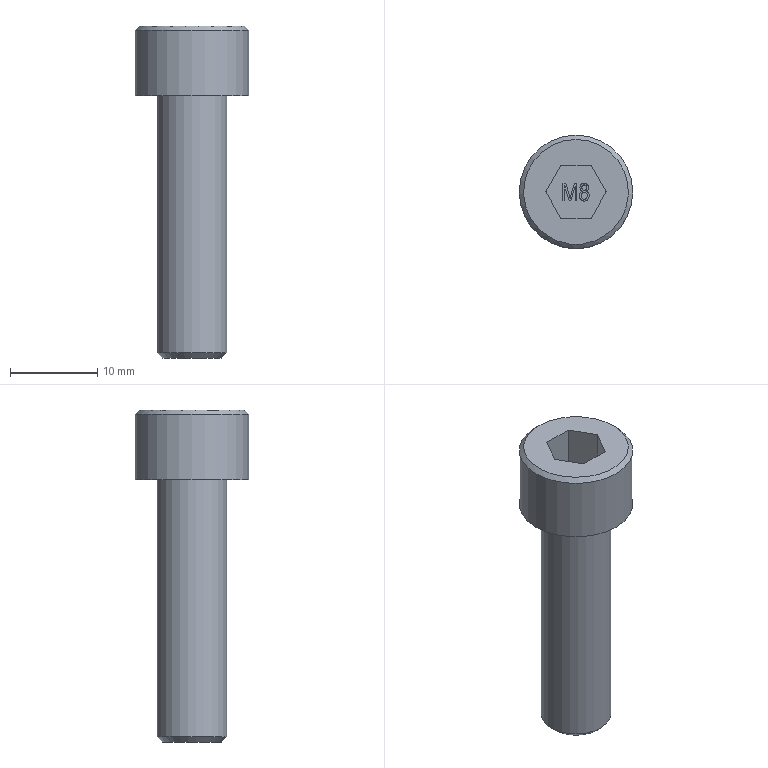Part | STEP file | EM10803000 | 1 solid | 38 faces | box 13 x 13 x 38 mm | volume 2405 mm3 | plane 25 | other 9 | cylinder 2 | cone 2 | commonest cylinder face diameters 8 x1 13 x1